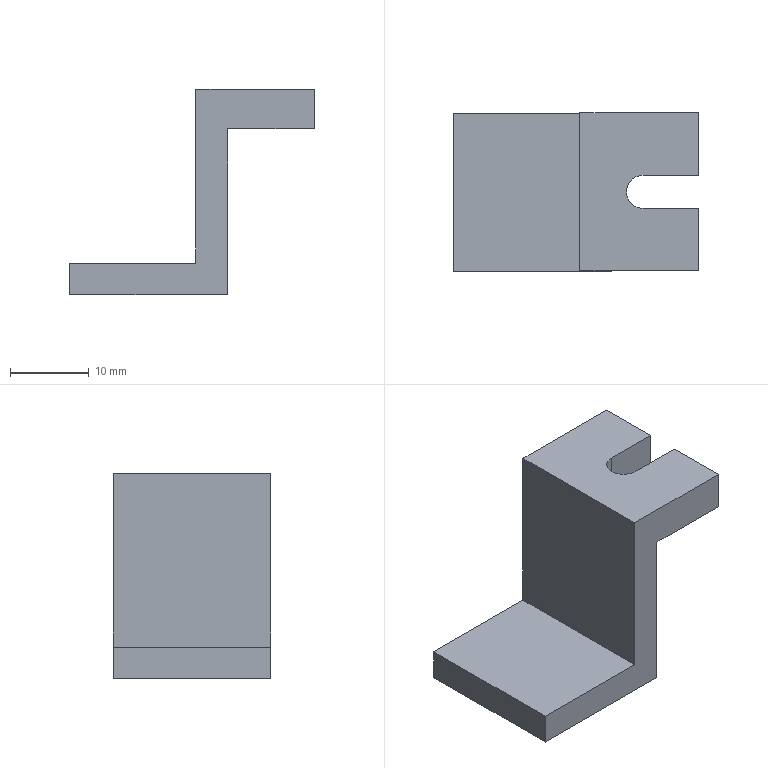Part | SolidWorks | features Extrusion 1, ICE 1 | 1 solid | 15 faces | box 31 x 20 x 26 mm | volume 4278 mm3 | plane 13 | cylinder 2 | commonest cylinder face diameters 4.2 x2
STEP:
#1=CARTESIAN_POINT('',(1.426,12.1,17.347));
#2=VERTEX_POINT('',#1);
#3=CARTESIAN_POINT('',(-0.6743,10.,17.347));
#4=VERTEX_POINT('',#3);
#5=CARTESIAN_POINT('',(1.426,10.,17.347));
#6=DIRECTION('',(0.,0.,1.));
#7=DIRECTION('',(1.,0.,0.));
#8=AXIS2_PLACEMENT_3D('',#5,#6,#7);
#9=CIRCLE('',#8,2.1);
#10=EDGE_CURVE('',#2,#4,#9,.T.);
#11=ORIENTED_EDGE('',*,*,#10,.T.);
#12=CARTESIAN_POINT('',(-0.6743,10.,12.347));
#13=VERTEX_POINT('',#12);
#14=CARTESIAN_POINT('',(-0.6743,10.,27.347));
#15=DIRECTION('',(0.,0.,-1.));
#16=VECTOR('',#15,1000.);
#17=LINE('',#14,#16);
#18=EDGE_CURVE('',#4,#13,#17,.T.);
#19=ORIENTED_EDGE('',*,*,#18,.T.);
#20=CARTESIAN_POINT('',(1.426,12.1,12.347));
#21=VERTEX_POINT('',#20);
#22=CARTESIAN_POINT('',(1.426,10.,12.347));
#23=DIRECTION('',(0.,0.,-1.));
#24=DIRECTION('',(-1.,0.,0.));
#25=AXIS2_PLACEMENT_3D('',#22,#23,#24);
#26=CIRCLE('',#25,2.1);
#27=EDGE_CURVE('',#13,#21,#26,.T.);
#28=ORIENTED_EDGE('',*,*,#27,.T.);
#29=CARTESIAN_POINT('',(1.426,12.1,27.347));
#30=DIRECTION('',(0.,0.,-1.));
#31=VECTOR('',#30,1000.);
#32=LINE('',#29,#31);
#33=EDGE_CURVE('',#2,#21,#32,.T.);
#34=ORIENTED_EDGE('',*,*,#33,.F.);
#35=EDGE_LOOP('',(#11,#19,#28,#34));
#36=FACE_OUTER_BOUND('',#35,.T.);
#37=CARTESIAN_POINT('',(1.426,10.,27.347));
#38=DIRECTION('',(0.,0.,-1.));
#39=DIRECTION('',(-1.,0.,0.));
#40=AXIS2_PLACEMENT_3D('',#37,#38,#39);
#41=CYLINDRICAL_SURFACE('',#40,2.1);
#42=ADVANCED_FACE('',(#36),#41,.F.);
#43=CARTESIAN_POINT('',(8.426,7.9,12.347));
#44=VERTEX_POINT('',#43);
#45=CARTESIAN_POINT('',(8.426,0.,12.347));
#46=VERTEX_POINT('',#45);
#47=CARTESIAN_POINT('',(8.426,20.,12.347));
#48=DIRECTION('',(0.,-1.,0.));
#49=VECTOR('',#48,1000.);
#50=LINE('',#47,#49);
#51=EDGE_CURVE('',#44,#46,#50,.T.);
#52=ORIENTED_EDGE('',*,*,#51,.F.);
#53=CARTESIAN_POINT('',(8.426,7.9,17.347));
#54=VERTEX_POINT('',#53);
#55=CARTESIAN_POINT('',(8.426,7.9,0.));
#56=DIRECTION('',(0.,0.,1.));
#57=VECTOR('',#56,1000.);
#58=LINE('',#55,#57);
#59=EDGE_CURVE('',#44,#54,#58,.T.);
#60=ORIENTED_EDGE('',*,*,#59,.T.);
#61=CARTESIAN_POINT('',(8.426,0.,17.347));
#62=VERTEX_POINT('',#61);
#63=CARTESIAN_POINT('',(8.426,20.,17.347));
#64=DIRECTION('',(0.,-1.,0.));
#65=VECTOR('',#64,1000.);
#66=LINE('',#63,#65);
#67=EDGE_CURVE('',#54,#62,#66,.T.);
#68=ORIENTED_EDGE('',*,*,#67,.T.);
#69=CARTESIAN_POINT('',(8.426,0.,0.));
#70=DIRECTION('',(0.,0.,-1.));
#71=VECTOR('',#70,1000.);
#72=LINE('',#69,#71);
#73=EDGE_CURVE('',#62,#46,#72,.T.);
#74=ORIENTED_EDGE('',*,*,#73,.T.);
#75=EDGE_LOOP('',(#52,#60,#68,#74));
#76=FACE_OUTER_BOUND('',#75,.T.);
#77=CARTESIAN_POINT('',(8.426,20.,0.));
#78=DIRECTION('',(-1.,0.,0.));
#79=DIRECTION('',(0.,0.,1.));
#80=AXIS2_PLACEMENT_3D('',#77,#78,#79);
#81=PLANE('',#80);
#82=ADVANCED_FACE('',(#76),#81,.F.);
#83=CARTESIAN_POINT('',(-22.574,0.,-4.653));
#84=VERTEX_POINT('',#83);
#85=CARTESIAN_POINT('',(-6.574,0.,-4.653));
#86=VERTEX_POINT('',#85);
#87=CARTESIAN_POINT('',(0.,0.,-4.653));
#88=DIRECTION('',(1.,0.,0.));
#89=VECTOR('',#88,1000.);
#90=LINE('',#87,#89);
#91=EDGE_CURVE('',#84,#86,#90,.T.);
#92=ORIENTED_EDGE('',*,*,#91,.T.);
#93=CARTESIAN_POINT('',(-6.574,20.,-4.653));
#94=VERTEX_POINT('',#93);
#95=CARTESIAN_POINT('',(-6.574,20.,-4.653));
#96=DIRECTION('',(0.,-1.,0.));
#97=VECTOR('',#96,1000.);
#98=LINE('',#95,#97);
#99=EDGE_CURVE('',#94,#86,#98,.T.);
#100=ORIENTED_EDGE('',*,*,#99,.F.);
#101=CARTESIAN_POINT('',(-22.574,20.,-4.653));
#102=VERTEX_POINT('',#101);
#103=CARTESIAN_POINT('',(0.,20.,-4.653));
#104=DIRECTION('',(1.,0.,0.));
#105=VECTOR('',#104,1000.);
#106=LINE('',#103,#105);
#107=EDGE_CURVE('',#102,#94,#106,.T.);
#108=ORIENTED_EDGE('',*,*,#107,.F.);
#109=CARTESIAN_POINT('',(-22.574,20.,-4.653));
#110=DIRECTION('',(0.,-1.,0.));
#111=VECTOR('',#110,1000.);
#112=LINE('',#109,#111);
#113=EDGE_CURVE('',#102,#84,#112,.T.);
#114=ORIENTED_EDGE('',*,*,#113,.T.);
#115=EDGE_LOOP('',(#92,#100,#108,#114));
#116=FACE_OUTER_BOUND('',#115,.T.);
#117=CARTESIAN_POINT('',(0.,20.,-4.653));
#118=DIRECTION('',(0.,0.,-1.));
#119=DIRECTION('',(-1.,0.,0.));
#120=AXIS2_PLACEMENT_3D('',#117,#118,#119);
#121=PLANE('',#120);
#122=ADVANCED_FACE('',(#116),#121,.F.);
#123=CARTESIAN_POINT('',(-6.574,0.,17.347));
#124=VERTEX_POINT('',#123);
#125=CARTESIAN_POINT('',(-6.574,0.,0.));
#126=DIRECTION('',(0.,0.,1.));
#127=VECTOR('',#126,1000.);
#128=LINE('',#125,#127);
#129=EDGE_CURVE('',#86,#124,#128,.T.);
#130=ORIENTED_EDGE('',*,*,#129,.T.);
#131=CARTESIAN_POINT('',(-6.574,20.,17.347));
#132=VERTEX_POINT('',#131);
#133=CARTESIAN_POINT('',(-6.574,20.,17.347));
#134=DIRECTION('',(0.,-1.,0.));
#135=VECTOR('',#134,1000.);
#136=LINE('',#133,#135);
#137=EDGE_CURVE('',#132,#124,#136,.T.);
#138=ORIENTED_EDGE('',*,*,#137,.F.);
#139=CARTESIAN_POINT('',(-6.574,20.,0.));
#140=DIRECTION('',(0.,0.,1.));
#141=VECTOR('',#140,1000.);
#142=LINE('',#139,#141);
#143=EDGE_CURVE('',#94,#132,#142,.T.);
#144=ORIENTED_EDGE('',*,*,#143,.F.);
#145=ORIENTED_EDGE('',*,*,#99,.T.);
#146=EDGE_LOOP('',(#130,#138,#144,#145));
#147=FACE_OUTER_BOUND('',#146,.T.);
#148=CARTESIAN_POINT('',(-6.574,20.,0.));
#149=DIRECTION('',(1.,0.,0.));
#150=DIRECTION('',(0.,0.,-1.));
#151=AXIS2_PLACEMENT_3D('',#148,#149,#150);
#152=PLANE('',#151);
#153=ADVANCED_FACE('',(#147),#152,.F.);
#154=CARTESIAN_POINT('',(1.426,7.9,17.347));
#155=VERTEX_POINT('',#154);
#156=CARTESIAN_POINT('',(0.,7.9,17.347));
#157=DIRECTION('',(1.,0.,0.));
#158=VECTOR('',#157,1000.);
#159=LINE('',#156,#158);
#160=EDGE_CURVE('',#155,#54,#159,.T.);
#161=ORIENTED_EDGE('',*,*,#160,.F.);
#162=CARTESIAN_POINT('',(1.426,10.,17.347));
#163=DIRECTION('',(0.,0.,1.));
#164=DIRECTION('',(1.,0.,0.));
#165=AXIS2_PLACEMENT_3D('',#162,#163,#164);
#166=CIRCLE('',#165,2.1);
#167=EDGE_CURVE('',#4,#155,#166,.T.);
#168=ORIENTED_EDGE('',*,*,#167,.F.);
#169=ORIENTED_EDGE('',*,*,#10,.F.);
#170=CARTESIAN_POINT('',(8.426,12.1,17.347));
#171=VERTEX_POINT('',#170);
#172=CARTESIAN_POINT('',(0.,12.1,17.347));
#173=DIRECTION('',(-1.,0.,0.));
#174=VECTOR('',#173,1000.);
#175=LINE('',#172,#174);
#176=EDGE_CURVE('',#171,#2,#175,.T.);
#177=ORIENTED_EDGE('',*,*,#176,.F.);
#178=CARTESIAN_POINT('',(8.426,20.,17.347));
#179=VERTEX_POINT('',#178);
#180=CARTESIAN_POINT('',(8.426,20.,17.347));
#181=DIRECTION('',(0.,-1.,0.));
#182=VECTOR('',#181,1000.);
#183=LINE('',#180,#182);
#184=EDGE_CURVE('',#179,#171,#183,.T.);
#185=ORIENTED_EDGE('',*,*,#184,.F.);
#186=CARTESIAN_POINT('',(0.,20.,17.347));
#187=DIRECTION('',(-1.,0.,0.));
#188=VECTOR('',#187,1000.);
#189=LINE('',#186,#188);
#190=EDGE_CURVE('',#179,#132,#189,.T.);
#191=ORIENTED_EDGE('',*,*,#190,.T.);
#192=ORIENTED_EDGE('',*,*,#137,.T.);
#193=CARTESIAN_POINT('',(0.,0.,17.347));
#194=DIRECTION('',(-1.,0.,0.));
#195=VECTOR('',#194,1000.);
#196=LINE('',#193,#195);
#197=EDGE_CURVE('',#62,#124,#196,.T.);
#198=ORIENTED_EDGE('',*,*,#197,.F.);
#199=ORIENTED_EDGE('',*,*,#67,.F.);
#200=EDGE_LOOP('',(#161,#168,#169,#177,#185,#191,#192,#198,#199));
#201=FACE_OUTER_BOUND('',#200,.T.);
#202=CARTESIAN_POINT('',(0.,20.,17.347));
#203=DIRECTION('',(0.,0.,1.));
#204=DIRECTION('',(1.,0.,0.));
#205=AXIS2_PLACEMENT_3D('',#202,#203,#204);
#206=PLANE('',#205);
#207=ADVANCED_FACE('',(#201),#206,.T.);
#208=ORIENTED_EDGE('',*,*,#184,.T.);
#209=CARTESIAN_POINT('',(8.426,12.1,12.347));
#210=VERTEX_POINT('',#209);
#211=CARTESIAN_POINT('',(8.426,12.1,0.));
#212=DIRECTION('',(0.,0.,-1.));
#213=VECTOR('',#212,1000.);
#214=LINE('',#211,#213);
#215=EDGE_CURVE('',#171,#210,#214,.T.);
#216=ORIENTED_EDGE('',*,*,#215,.T.);
#217=CARTESIAN_POINT('',(8.426,20.,12.347));
#218=VERTEX_POINT('',#217);
#219=CARTESIAN_POINT('',(8.426,20.,12.347));
#220=DIRECTION('',(0.,-1.,0.));
#221=VECTOR('',#220,1000.);
#222=LINE('',#219,#221);
#223=EDGE_CURVE('',#218,#210,#222,.T.);
#224=ORIENTED_EDGE('',*,*,#223,.F.);
#225=CARTESIAN_POINT('',(8.426,20.,0.));
#226=DIRECTION('',(0.,0.,-1.));
#227=VECTOR('',#226,1000.);
#228=LINE('',#225,#227);
#229=EDGE_CURVE('',#179,#218,#228,.T.);
#230=ORIENTED_EDGE('',*,*,#229,.F.);
#231=EDGE_LOOP('',(#208,#216,#224,#230));
#232=FACE_OUTER_BOUND('',#231,.T.);
#233=CARTESIAN_POINT('',(8.426,20.,0.));
#234=DIRECTION('',(-1.,0.,0.));
#235=DIRECTION('',(0.,0.,1.));
#236=AXIS2_PLACEMENT_3D('',#233,#234,#235);
#237=PLANE('',#236);
#238=ADVANCED_FACE('',(#232),#237,.F.);
#239=CARTESIAN_POINT('',(1.426,7.9,12.347));
#240=VERTEX_POINT('',#239);
#241=CARTESIAN_POINT('',(0.,7.9,12.347));
#242=DIRECTION('',(-1.,0.,0.));
#243=VECTOR('',#242,1000.);
#244=LINE('',#241,#243);
#245=EDGE_CURVE('',#44,#240,#244,.T.);
#246=ORIENTED_EDGE('',*,*,#245,.F.);
#247=ORIENTED_EDGE('',*,*,#51,.T.);
#248=CARTESIAN_POINT('',(-2.574,0.,12.347));
#249=VERTEX_POINT('',#248);
#250=CARTESIAN_POINT('',(0.,0.,12.347));
#251=DIRECTION('',(1.,0.,0.));
#252=VECTOR('',#251,1000.);
#253=LINE('',#250,#252);
#254=EDGE_CURVE('',#249,#46,#253,.T.);
#255=ORIENTED_EDGE('',*,*,#254,.F.);
#256=CARTESIAN_POINT('',(-2.574,20.,12.347));
#257=VERTEX_POINT('',#256);
#258=CARTESIAN_POINT('',(-2.574,20.,12.347));
#259=DIRECTION('',(0.,-1.,0.));
#260=VECTOR('',#259,1000.);
#261=LINE('',#258,#260);
#262=EDGE_CURVE('',#257,#249,#261,.T.);
#263=ORIENTED_EDGE('',*,*,#262,.F.);
#264=CARTESIAN_POINT('',(0.,20.,12.347));
#265=DIRECTION('',(1.,0.,0.));
#266=VECTOR('',#265,1000.);
#267=LINE('',#264,#266);
#268=EDGE_CURVE('',#257,#218,#267,.T.);
#269=ORIENTED_EDGE('',*,*,#268,.T.);
#270=ORIENTED_EDGE('',*,*,#223,.T.);
#271=CARTESIAN_POINT('',(5.426,12.1,12.347));
#272=DIRECTION('',(1.,0.,0.));
#273=VECTOR('',#272,1000.);
#274=LINE('',#271,#273);
#275=EDGE_CURVE('',#21,#210,#274,.T.);
#276=ORIENTED_EDGE('',*,*,#275,.F.);
#277=ORIENTED_EDGE('',*,*,#27,.F.);
#278=CARTESIAN_POINT('',(1.426,10.,12.347));
#279=DIRECTION('',(0.,0.,-1.));
#280=DIRECTION('',(-1.,0.,0.));
#281=AXIS2_PLACEMENT_3D('',#278,#279,#280);
#282=CIRCLE('',#281,2.1);
#283=EDGE_CURVE('',#240,#13,#282,.T.);
#284=ORIENTED_EDGE('',*,*,#283,.F.);
#285=EDGE_LOOP('',(#246,#247,#255,#263,#269,#270,#276,#277,#284));
#286=FACE_OUTER_BOUND('',#285,.T.);
#287=CARTESIAN_POINT('',(0.,20.,12.347));
#288=DIRECTION('',(0.,0.,-1.));
#289=DIRECTION('',(-1.,0.,0.));
#290=AXIS2_PLACEMENT_3D('',#287,#288,#289);
#291=PLANE('',#290);
#292=ADVANCED_FACE('',(#286),#291,.T.);
#293=CARTESIAN_POINT('',(-2.574,0.,-8.653));
#294=VERTEX_POINT('',#293);
#295=CARTESIAN_POINT('',(-2.574,0.,0.));
#296=DIRECTION('',(0.,0.,1.));
#297=VECTOR('',#296,1000.);
#298=LINE('',#295,#297);
#299=EDGE_CURVE('',#294,#249,#298,.T.);
#300=ORIENTED_EDGE('',*,*,#299,.F.);
#301=CARTESIAN_POINT('',(-2.574,20.,-8.653));
#302=VERTEX_POINT('',#301);
#303=CARTESIAN_POINT('',(-2.574,20.,-8.653));
#304=DIRECTION('',(0.,-1.,0.));
#305=VECTOR('',#304,1000.);
#306=LINE('',#303,#305);
#307=EDGE_CURVE('',#302,#294,#306,.T.);
#308=ORIENTED_EDGE('',*,*,#307,.F.);
#309=CARTESIAN_POINT('',(-2.574,20.,0.));
#310=DIRECTION('',(0.,0.,1.));
#311=VECTOR('',#310,1000.);
#312=LINE('',#309,#311);
#313=EDGE_CURVE('',#302,#257,#312,.T.);
#314=ORIENTED_EDGE('',*,*,#313,.T.);
#315=ORIENTED_EDGE('',*,*,#262,.T.);
#316=EDGE_LOOP('',(#300,#308,#314,#315));
#317=FACE_OUTER_BOUND('',#316,.T.);
#318=CARTESIAN_POINT('',(-2.574,20.,0.));
#319=DIRECTION('',(1.,0.,0.));
#320=DIRECTION('',(0.,0.,-1.));
#321=AXIS2_PLACEMENT_3D('',#318,#319,#320);
#322=PLANE('',#321);
#323=ADVANCED_FACE('',(#317),#322,.T.);
#324=CARTESIAN_POINT('',(-22.574,0.,-8.653));
#325=VERTEX_POINT('',#324);
#326=CARTESIAN_POINT('',(0.,0.,-8.653));
#327=DIRECTION('',(1.,0.,0.));
#328=VECTOR('',#327,1000.);
#329=LINE('',#326,#328);
#330=EDGE_CURVE('',#325,#294,#329,.T.);
#331=ORIENTED_EDGE('',*,*,#330,.F.);
#332=CARTESIAN_POINT('',(-22.574,20.,-8.653));
#333=VERTEX_POINT('',#332);
#334=CARTESIAN_POINT('',(-22.574,20.,-8.653));
#335=DIRECTION('',(0.,-1.,0.));
#336=VECTOR('',#335,1000.);
#337=LINE('',#334,#336);
#338=EDGE_CURVE('',#333,#325,#337,.T.);
#339=ORIENTED_EDGE('',*,*,#338,.F.);
#340=CARTESIAN_POINT('',(0.,20.,-8.653));
#341=DIRECTION('',(1.,0.,0.));
#342=VECTOR('',#341,1000.);
#343=LINE('',#340,#342);
#344=EDGE_CURVE('',#333,#302,#343,.T.);
#345=ORIENTED_EDGE('',*,*,#344,.T.);
#346=ORIENTED_EDGE('',*,*,#307,.T.);
#347=EDGE_LOOP('',(#331,#339,#345,#346));
#348=FACE_OUTER_BOUND('',#347,.T.);
#349=CARTESIAN_POINT('',(0.,20.,-8.653));
#350=DIRECTION('',(0.,0.,-1.));
#351=DIRECTION('',(-1.,0.,0.));
#352=AXIS2_PLACEMENT_3D('',#349,#350,#351);
#353=PLANE('',#352);
#354=ADVANCED_FACE('',(#348),#353,.T.);
#355=CARTESIAN_POINT('',(-22.574,0.,0.));
#356=DIRECTION('',(0.,0.,1.));
#357=VECTOR('',#356,1000.);
#358=LINE('',#355,#357);
#359=EDGE_CURVE('',#325,#84,#358,.T.);
#360=ORIENTED_EDGE('',*,*,#359,.T.);
#361=ORIENTED_EDGE('',*,*,#113,.F.);
#362=CARTESIAN_POINT('',(-22.574,20.,0.));
#363=DIRECTION('',(0.,0.,1.));
#364=VECTOR('',#363,1000.);
#365=LINE('',#362,#364);
#366=EDGE_CURVE('',#333,#102,#365,.T.);
#367=ORIENTED_EDGE('',*,*,#366,.F.);
#368=ORIENTED_EDGE('',*,*,#338,.T.);
#369=EDGE_LOOP('',(#360,#361,#367,#368));
#370=FACE_OUTER_BOUND('',#369,.T.);
#371=CARTESIAN_POINT('',(-22.574,20.,0.));
#372=DIRECTION('',(1.,0.,0.));
#373=DIRECTION('',(0.,0.,-1.));
#374=AXIS2_PLACEMENT_3D('',#371,#372,#373);
#375=PLANE('',#374);
#376=ADVANCED_FACE('',(#370),#375,.F.);
#377=ORIENTED_EDGE('',*,*,#107,.T.);
#378=ORIENTED_EDGE('',*,*,#143,.T.);
#379=ORIENTED_EDGE('',*,*,#190,.F.);
#380=ORIENTED_EDGE('',*,*,#229,.T.);
#381=ORIENTED_EDGE('',*,*,#268,.F.);
#382=ORIENTED_EDGE('',*,*,#313,.F.);
#383=ORIENTED_EDGE('',*,*,#344,.F.);
#384=ORIENTED_EDGE('',*,*,#366,.T.);
#385=EDGE_LOOP('',(#377,#378,#379,#380,#381,#382,#383,#384));
#386=FACE_OUTER_BOUND('',#385,.T.);
#387=CARTESIAN_POINT('',(0.,20.,0.));
#388=DIRECTION('',(0.,1.,0.));
#389=DIRECTION('',(0.,0.,1.));
#390=AXIS2_PLACEMENT_3D('',#387,#388,#389);
#391=PLANE('',#390);
#392=ADVANCED_FACE('',(#386),#391,.T.);
#393=ORIENTED_EDGE('',*,*,#91,.F.);
#394=ORIENTED_EDGE('',*,*,#359,.F.);
#395=ORIENTED_EDGE('',*,*,#330,.T.);
#396=ORIENTED_EDGE('',*,*,#299,.T.);
#397=ORIENTED_EDGE('',*,*,#254,.T.);
#398=ORIENTED_EDGE('',*,*,#73,.F.);
#399=ORIENTED_EDGE('',*,*,#197,.T.);
#400=ORIENTED_EDGE('',*,*,#129,.F.);
#401=EDGE_LOOP('',(#393,#394,#395,#396,#397,#398,#399,#400));
#402=FACE_OUTER_BOUND('',#401,.T.);
#403=CARTESIAN_POINT('',(0.,0.,0.));
#404=DIRECTION('',(0.,1.,0.));
#405=DIRECTION('',(0.,0.,1.));
#406=AXIS2_PLACEMENT_3D('',#403,#404,#405);
#407=PLANE('',#406);
#408=ADVANCED_FACE('',(#402),#407,.F.);
#409=ORIENTED_EDGE('',*,*,#160,.T.);
#410=ORIENTED_EDGE('',*,*,#59,.F.);
#411=ORIENTED_EDGE('',*,*,#245,.T.);
#412=CARTESIAN_POINT('',(1.426,7.9,27.347));
#413=DIRECTION('',(0.,0.,-1.));
#414=VECTOR('',#413,1000.);
#415=LINE('',#412,#414);
#416=EDGE_CURVE('',#155,#240,#415,.T.);
#417=ORIENTED_EDGE('',*,*,#416,.F.);
#418=EDGE_LOOP('',(#409,#410,#411,#417));
#419=FACE_OUTER_BOUND('',#418,.T.);
#420=CARTESIAN_POINT('',(5.426,7.9,27.347));
#421=DIRECTION('',(0.,-1.,0.));
#422=DIRECTION('',(0.,0.,-1.));
#423=AXIS2_PLACEMENT_3D('',#420,#421,#422);
#424=PLANE('',#423);
#425=ADVANCED_FACE('',(#419),#424,.F.);
#426=ORIENTED_EDGE('',*,*,#176,.T.);
#427=ORIENTED_EDGE('',*,*,#33,.T.);
#428=ORIENTED_EDGE('',*,*,#275,.T.);
#429=ORIENTED_EDGE('',*,*,#215,.F.);
#430=EDGE_LOOP('',(#426,#427,#428,#429));
#431=FACE_OUTER_BOUND('',#430,.T.);
#432=CARTESIAN_POINT('',(5.426,12.1,27.347));
#433=DIRECTION('',(0.,1.,0.));
#434=DIRECTION('',(0.,0.,1.));
#435=AXIS2_PLACEMENT_3D('',#432,#433,#434);
#436=PLANE('',#435);
#437=ADVANCED_FACE('',(#431),#436,.F.);
#438=ORIENTED_EDGE('',*,*,#18,.F.);
#439=ORIENTED_EDGE('',*,*,#167,.T.);
#440=ORIENTED_EDGE('',*,*,#416,.T.);
#441=ORIENTED_EDGE('',*,*,#283,.T.);
#442=EDGE_LOOP('',(#438,#439,#440,#441));
#443=FACE_OUTER_BOUND('',#442,.T.);
#444=CARTESIAN_POINT('',(1.426,10.,27.347));
#445=DIRECTION('',(0.,0.,-1.));
#446=DIRECTION('',(-1.,0.,0.));
#447=AXIS2_PLACEMENT_3D('',#444,#445,#446);
#448=CYLINDRICAL_SURFACE('',#447,2.1);
#449=ADVANCED_FACE('',(#443),#448,.F.);
#450=CLOSED_SHELL('',(#42,#82,#122,#153,#207,#238,#292,#323,#354,#376,#392,#408,#425,#437,#449));
#451=MANIFOLD_SOLID_BREP('',#450);
#452=CARTESIAN_POINT('',(0.,0.,0.));
#453=DIRECTION('',(0.,0.,1.));
#454=DIRECTION('',(1.,0.,0.));
#455=AXIS2_PLACEMENT_3D('',#452,#453,#454);
#456=(LENGTH_UNIT()NAMED_UNIT(*)SI_UNIT(.MILLI.,.METRE.));
#457=UNCERTAINTY_MEASURE_WITH_UNIT(LENGTH_MEASURE(0.00001),#456,'','');
#458=(NAMED_UNIT(*)PLANE_ANGLE_UNIT()SI_UNIT($,.RADIAN.));
#459=(NAMED_UNIT(*)SI_UNIT($,.STERADIAN.)SOLID_ANGLE_UNIT());
#460=(GEOMETRIC_REPRESENTATION_CONTEXT(3)GLOBAL_UNCERTAINTY_ASSIGNED_CONTEXT((#457))GLOBAL_UNIT_ASSIGNED_CONTEXT((#456,#458,#459))REPRESENTATION_CONTEXT('',''));
#461=ADVANCED_BREP_SHAPE_REPRESENTATION('',(#451,#455),#460);